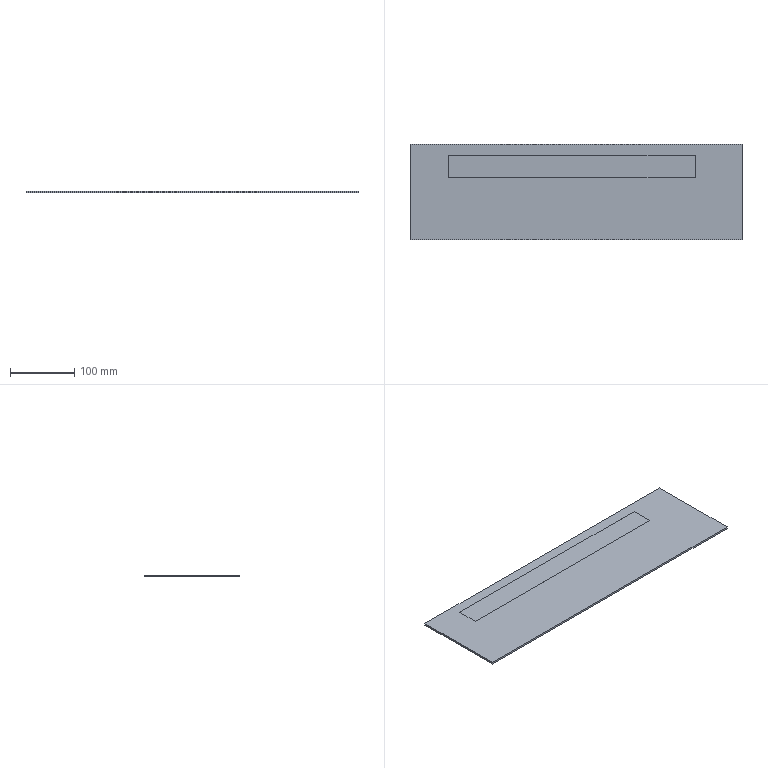Part | SolidWorks | features Extrusion 1, ICE 1 | 1 solid | 11 faces | box 515 x 148 x 3.01 mm | volume 228793 mm3 | plane 11
STEP:
#1=CARTESIAN_POINT('',(257.5,-74.,3.));
#2=VERTEX_POINT('',#1);
#3=CARTESIAN_POINT('',(257.5,74.,3.));
#4=VERTEX_POINT('',#3);
#5=CARTESIAN_POINT('',(257.5,74.,3.));
#6=DIRECTION('',(0.,1.,0.));
#7=VECTOR('',#6,1000.);
#8=LINE('',#5,#7);
#9=EDGE_CURVE('',#2,#4,#8,.T.);
#10=ORIENTED_EDGE('',*,*,#9,.T.);
#11=CARTESIAN_POINT('',(-257.5,74.,3.));
#12=VERTEX_POINT('',#11);
#13=CARTESIAN_POINT('',(-257.5,74.,3.));
#14=DIRECTION('',(-1.,0.,0.));
#15=VECTOR('',#14,1000.);
#16=LINE('',#13,#15);
#17=EDGE_CURVE('',#4,#12,#16,.T.);
#18=ORIENTED_EDGE('',*,*,#17,.T.);
#19=CARTESIAN_POINT('',(-257.5,-74.,3.));
#20=VERTEX_POINT('',#19);
#21=CARTESIAN_POINT('',(-257.5,74.,3.));
#22=DIRECTION('',(0.,-1.,0.));
#23=VECTOR('',#22,1000.);
#24=LINE('',#21,#23);
#25=EDGE_CURVE('',#12,#20,#24,.T.);
#26=ORIENTED_EDGE('',*,*,#25,.T.);
#27=CARTESIAN_POINT('',(-257.5,-74.,3.));
#28=DIRECTION('',(1.,0.,0.));
#29=VECTOR('',#28,1000.);
#30=LINE('',#27,#29);
#31=EDGE_CURVE('',#20,#2,#30,.T.);
#32=ORIENTED_EDGE('',*,*,#31,.T.);
#33=EDGE_LOOP('',(#10,#18,#26,#32));
#34=FACE_OUTER_BOUND('',#33,.T.);
#35=CARTESIAN_POINT('',(184.856,57.328,3.));
#36=VERTEX_POINT('',#35);
#37=CARTESIAN_POINT('',(-198.111,57.328,3.));
#38=VERTEX_POINT('',#37);
#39=CARTESIAN_POINT('',(184.856,57.328,3.));
#40=DIRECTION('',(-1.,0.,0.));
#41=VECTOR('',#40,1000.);
#42=LINE('',#39,#41);
#43=EDGE_CURVE('',#36,#38,#42,.T.);
#44=ORIENTED_EDGE('',*,*,#43,.F.);
#45=CARTESIAN_POINT('',(184.856,22.632,3.));
#46=VERTEX_POINT('',#45);
#47=CARTESIAN_POINT('',(184.856,57.328,3.));
#48=DIRECTION('',(0.,1.,0.));
#49=VECTOR('',#48,1000.);
#50=LINE('',#47,#49);
#51=EDGE_CURVE('',#46,#36,#50,.T.);
#52=ORIENTED_EDGE('',*,*,#51,.F.);
#53=CARTESIAN_POINT('',(-198.111,22.632,3.));
#54=VERTEX_POINT('',#53);
#55=CARTESIAN_POINT('',(184.856,22.632,3.));
#56=DIRECTION('',(1.,0.,0.));
#57=VECTOR('',#56,1000.);
#58=LINE('',#55,#57);
#59=EDGE_CURVE('',#54,#46,#58,.T.);
#60=ORIENTED_EDGE('',*,*,#59,.F.);
#61=CARTESIAN_POINT('',(-198.111,57.328,3.));
#62=DIRECTION('',(0.,-1.,0.));
#63=VECTOR('',#62,1000.);
#64=LINE('',#61,#63);
#65=EDGE_CURVE('',#38,#54,#64,.T.);
#66=ORIENTED_EDGE('',*,*,#65,.F.);
#67=EDGE_LOOP('',(#44,#52,#60,#66));
#68=FACE_BOUND('',#67,.T.);
#69=CARTESIAN_POINT('',(0.,0.,3.));
#70=DIRECTION('',(0.,0.,1.));
#71=DIRECTION('',(1.,0.,0.));
#72=AXIS2_PLACEMENT_3D('',#69,#70,#71);
#73=PLANE('',#72);
#74=ADVANCED_FACE('',(#34,#68),#73,.T.);
#75=CARTESIAN_POINT('',(257.5,-74.,0.));
#76=VERTEX_POINT('',#75);
#77=CARTESIAN_POINT('',(257.5,74.,0.));
#78=VERTEX_POINT('',#77);
#79=CARTESIAN_POINT('',(257.5,74.,0.));
#80=DIRECTION('',(0.,1.,0.));
#81=VECTOR('',#80,1000.);
#82=LINE('',#79,#81);
#83=EDGE_CURVE('',#76,#78,#82,.T.);
#84=ORIENTED_EDGE('',*,*,#83,.T.);
#85=CARTESIAN_POINT('',(257.5,74.,3.));
#86=DIRECTION('',(0.,0.,-1.));
#87=VECTOR('',#86,1000.);
#88=LINE('',#85,#87);
#89=EDGE_CURVE('',#4,#78,#88,.T.);
#90=ORIENTED_EDGE('',*,*,#89,.F.);
#91=ORIENTED_EDGE('',*,*,#9,.F.);
#92=CARTESIAN_POINT('',(257.5,-74.,3.));
#93=DIRECTION('',(0.,0.,-1.));
#94=VECTOR('',#93,1000.);
#95=LINE('',#92,#94);
#96=EDGE_CURVE('',#2,#76,#95,.T.);
#97=ORIENTED_EDGE('',*,*,#96,.T.);
#98=EDGE_LOOP('',(#84,#90,#91,#97));
#99=FACE_OUTER_BOUND('',#98,.T.);
#100=CARTESIAN_POINT('',(257.5,74.,3.));
#101=DIRECTION('',(-1.,0.,0.));
#102=DIRECTION('',(0.,0.,1.));
#103=AXIS2_PLACEMENT_3D('',#100,#101,#102);
#104=PLANE('',#103);
#105=ADVANCED_FACE('',(#99),#104,.F.);
#106=CARTESIAN_POINT('',(-257.5,74.,0.));
#107=VERTEX_POINT('',#106);
#108=CARTESIAN_POINT('',(-257.5,74.,0.));
#109=DIRECTION('',(-1.,0.,0.));
#110=VECTOR('',#109,1000.);
#111=LINE('',#108,#110);
#112=EDGE_CURVE('',#78,#107,#111,.T.);
#113=ORIENTED_EDGE('',*,*,#112,.T.);
#114=CARTESIAN_POINT('',(-257.5,74.,3.));
#115=DIRECTION('',(0.,0.,-1.));
#116=VECTOR('',#115,1000.);
#117=LINE('',#114,#116);
#118=EDGE_CURVE('',#12,#107,#117,.T.);
#119=ORIENTED_EDGE('',*,*,#118,.F.);
#120=ORIENTED_EDGE('',*,*,#17,.F.);
#121=ORIENTED_EDGE('',*,*,#89,.T.);
#122=EDGE_LOOP('',(#113,#119,#120,#121));
#123=FACE_OUTER_BOUND('',#122,.T.);
#124=CARTESIAN_POINT('',(-257.5,74.,3.));
#125=DIRECTION('',(0.,-1.,0.));
#126=DIRECTION('',(0.,0.,-1.));
#127=AXIS2_PLACEMENT_3D('',#124,#125,#126);
#128=PLANE('',#127);
#129=ADVANCED_FACE('',(#123),#128,.F.);
#130=CARTESIAN_POINT('',(-257.5,-74.,0.));
#131=VERTEX_POINT('',#130);
#132=CARTESIAN_POINT('',(-257.5,74.,0.));
#133=DIRECTION('',(0.,-1.,0.));
#134=VECTOR('',#133,1000.);
#135=LINE('',#132,#134);
#136=EDGE_CURVE('',#107,#131,#135,.T.);
#137=ORIENTED_EDGE('',*,*,#136,.T.);
#138=CARTESIAN_POINT('',(-257.5,-74.,3.));
#139=DIRECTION('',(0.,0.,-1.));
#140=VECTOR('',#139,1000.);
#141=LINE('',#138,#140);
#142=EDGE_CURVE('',#20,#131,#141,.T.);
#143=ORIENTED_EDGE('',*,*,#142,.F.);
#144=ORIENTED_EDGE('',*,*,#25,.F.);
#145=ORIENTED_EDGE('',*,*,#118,.T.);
#146=EDGE_LOOP('',(#137,#143,#144,#145));
#147=FACE_OUTER_BOUND('',#146,.T.);
#148=CARTESIAN_POINT('',(-257.5,74.,3.));
#149=DIRECTION('',(1.,0.,0.));
#150=DIRECTION('',(0.,0.,-1.));
#151=AXIS2_PLACEMENT_3D('',#148,#149,#150);
#152=PLANE('',#151);
#153=ADVANCED_FACE('',(#147),#152,.F.);
#154=CARTESIAN_POINT('',(-257.5,-74.,0.));
#155=DIRECTION('',(1.,0.,0.));
#156=VECTOR('',#155,1000.);
#157=LINE('',#154,#156);
#158=EDGE_CURVE('',#131,#76,#157,.T.);
#159=ORIENTED_EDGE('',*,*,#158,.T.);
#160=ORIENTED_EDGE('',*,*,#96,.F.);
#161=ORIENTED_EDGE('',*,*,#31,.F.);
#162=ORIENTED_EDGE('',*,*,#142,.T.);
#163=EDGE_LOOP('',(#159,#160,#161,#162));
#164=FACE_OUTER_BOUND('',#163,.T.);
#165=CARTESIAN_POINT('',(-257.5,-74.,3.));
#166=DIRECTION('',(0.,1.,0.));
#167=DIRECTION('',(0.,0.,1.));
#168=AXIS2_PLACEMENT_3D('',#165,#166,#167);
#169=PLANE('',#168);
#170=ADVANCED_FACE('',(#164),#169,.F.);
#171=ORIENTED_EDGE('',*,*,#83,.F.);
#172=ORIENTED_EDGE('',*,*,#158,.F.);
#173=ORIENTED_EDGE('',*,*,#136,.F.);
#174=ORIENTED_EDGE('',*,*,#112,.F.);
#175=EDGE_LOOP('',(#171,#172,#173,#174));
#176=FACE_OUTER_BOUND('',#175,.T.);
#177=CARTESIAN_POINT('',(0.,0.,0.));
#178=DIRECTION('',(0.,0.,1.));
#179=DIRECTION('',(1.,0.,0.));
#180=AXIS2_PLACEMENT_3D('',#177,#178,#179);
#181=PLANE('',#180);
#182=ADVANCED_FACE('',(#176),#181,.F.);
#183=ORIENTED_EDGE('',*,*,#51,.T.);
#184=CARTESIAN_POINT('',(184.856,57.328,3.01));
#185=VERTEX_POINT('',#184);
#186=CARTESIAN_POINT('',(184.856,57.328,3.01));
#187=DIRECTION('',(0.,0.,-1.));
#188=VECTOR('',#187,1000.);
#189=LINE('',#186,#188);
#190=EDGE_CURVE('',#185,#36,#189,.T.);
#191=ORIENTED_EDGE('',*,*,#190,.F.);
#192=CARTESIAN_POINT('',(184.856,22.632,3.01));
#193=VERTEX_POINT('',#192);
#194=CARTESIAN_POINT('',(184.856,57.328,3.01));
#195=DIRECTION('',(0.,1.,0.));
#196=VECTOR('',#195,1000.);
#197=LINE('',#194,#196);
#198=EDGE_CURVE('',#193,#185,#197,.T.);
#199=ORIENTED_EDGE('',*,*,#198,.F.);
#200=CARTESIAN_POINT('',(184.856,22.632,3.01));
#201=DIRECTION('',(0.,0.,-1.));
#202=VECTOR('',#201,1000.);
#203=LINE('',#200,#202);
#204=EDGE_CURVE('',#193,#46,#203,.T.);
#205=ORIENTED_EDGE('',*,*,#204,.T.);
#206=EDGE_LOOP('',(#183,#191,#199,#205));
#207=FACE_OUTER_BOUND('',#206,.T.);
#208=CARTESIAN_POINT('',(184.856,57.328,3.01));
#209=DIRECTION('',(-1.,0.,0.));
#210=DIRECTION('',(0.,0.,1.));
#211=AXIS2_PLACEMENT_3D('',#208,#209,#210);
#212=PLANE('',#211);
#213=ADVANCED_FACE('',(#207),#212,.F.);
#214=ORIENTED_EDGE('',*,*,#43,.T.);
#215=CARTESIAN_POINT('',(-198.111,57.328,3.01));
#216=VERTEX_POINT('',#215);
#217=CARTESIAN_POINT('',(-198.111,57.328,3.01));
#218=DIRECTION('',(0.,0.,-1.));
#219=VECTOR('',#218,1000.);
#220=LINE('',#217,#219);
#221=EDGE_CURVE('',#216,#38,#220,.T.);
#222=ORIENTED_EDGE('',*,*,#221,.F.);
#223=CARTESIAN_POINT('',(184.856,57.328,3.01));
#224=DIRECTION('',(-1.,0.,0.));
#225=VECTOR('',#224,1000.);
#226=LINE('',#223,#225);
#227=EDGE_CURVE('',#185,#216,#226,.T.);
#228=ORIENTED_EDGE('',*,*,#227,.F.);
#229=ORIENTED_EDGE('',*,*,#190,.T.);
#230=EDGE_LOOP('',(#214,#222,#228,#229));
#231=FACE_OUTER_BOUND('',#230,.T.);
#232=CARTESIAN_POINT('',(184.856,57.328,3.01));
#233=DIRECTION('',(0.,-1.,0.));
#234=DIRECTION('',(0.,0.,-1.));
#235=AXIS2_PLACEMENT_3D('',#232,#233,#234);
#236=PLANE('',#235);
#237=ADVANCED_FACE('',(#231),#236,.F.);
#238=ORIENTED_EDGE('',*,*,#65,.T.);
#239=CARTESIAN_POINT('',(-198.111,22.632,3.01));
#240=VERTEX_POINT('',#239);
#241=CARTESIAN_POINT('',(-198.111,22.632,3.01));
#242=DIRECTION('',(0.,0.,-1.));
#243=VECTOR('',#242,1000.);
#244=LINE('',#241,#243);
#245=EDGE_CURVE('',#240,#54,#244,.T.);
#246=ORIENTED_EDGE('',*,*,#245,.F.);
#247=CARTESIAN_POINT('',(-198.111,57.328,3.01));
#248=DIRECTION('',(0.,-1.,0.));
#249=VECTOR('',#248,1000.);
#250=LINE('',#247,#249);
#251=EDGE_CURVE('',#216,#240,#250,.T.);
#252=ORIENTED_EDGE('',*,*,#251,.F.);
#253=ORIENTED_EDGE('',*,*,#221,.T.);
#254=EDGE_LOOP('',(#238,#246,#252,#253));
#255=FACE_OUTER_BOUND('',#254,.T.);
#256=CARTESIAN_POINT('',(-198.111,57.328,3.01));
#257=DIRECTION('',(1.,0.,0.));
#258=DIRECTION('',(0.,0.,-1.));
#259=AXIS2_PLACEMENT_3D('',#256,#257,#258);
#260=PLANE('',#259);
#261=ADVANCED_FACE('',(#255),#260,.F.);
#262=ORIENTED_EDGE('',*,*,#59,.T.);
#263=ORIENTED_EDGE('',*,*,#204,.F.);
#264=CARTESIAN_POINT('',(184.856,22.632,3.01));
#265=DIRECTION('',(1.,0.,0.));
#266=VECTOR('',#265,1000.);
#267=LINE('',#264,#266);
#268=EDGE_CURVE('',#240,#193,#267,.T.);
#269=ORIENTED_EDGE('',*,*,#268,.F.);
#270=ORIENTED_EDGE('',*,*,#245,.T.);
#271=EDGE_LOOP('',(#262,#263,#269,#270));
#272=FACE_OUTER_BOUND('',#271,.T.);
#273=CARTESIAN_POINT('',(184.856,22.632,3.01));
#274=DIRECTION('',(0.,1.,0.));
#275=DIRECTION('',(0.,0.,1.));
#276=AXIS2_PLACEMENT_3D('',#273,#274,#275);
#277=PLANE('',#276);
#278=ADVANCED_FACE('',(#272),#277,.F.);
#279=ORIENTED_EDGE('',*,*,#198,.T.);
#280=ORIENTED_EDGE('',*,*,#227,.T.);
#281=ORIENTED_EDGE('',*,*,#251,.T.);
#282=ORIENTED_EDGE('',*,*,#268,.T.);
#283=EDGE_LOOP('',(#279,#280,#281,#282));
#284=FACE_OUTER_BOUND('',#283,.T.);
#285=CARTESIAN_POINT('',(0.,0.,3.01));
#286=DIRECTION('',(0.,0.,-1.));
#287=DIRECTION('',(-1.,0.,0.));
#288=AXIS2_PLACEMENT_3D('',#285,#286,#287);
#289=PLANE('',#288);
#290=ADVANCED_FACE('',(#284),#289,.F.);
#291=CLOSED_SHELL('',(#74,#105,#129,#153,#170,#182,#213,#237,#261,#278,#290));
#292=MANIFOLD_SOLID_BREP('',#291);
#293=CARTESIAN_POINT('',(0.,0.,0.));
#294=DIRECTION('',(0.,0.,1.));
#295=DIRECTION('',(1.,0.,0.));
#296=AXIS2_PLACEMENT_3D('',#293,#294,#295);
#297=(LENGTH_UNIT()NAMED_UNIT(*)SI_UNIT(.MILLI.,.METRE.));
#298=UNCERTAINTY_MEASURE_WITH_UNIT(LENGTH_MEASURE(0.00001),#297,'','');
#299=(NAMED_UNIT(*)PLANE_ANGLE_UNIT()SI_UNIT($,.RADIAN.));
#300=(NAMED_UNIT(*)SI_UNIT($,.STERADIAN.)SOLID_ANGLE_UNIT());
#301=(GEOMETRIC_REPRESENTATION_CONTEXT(3)GLOBAL_UNCERTAINTY_ASSIGNED_CONTEXT((#298))GLOBAL_UNIT_ASSIGNED_CONTEXT((#297,#299,#300))REPRESENTATION_CONTEXT('',''));
#302=ADVANCED_BREP_SHAPE_REPRESENTATION('',(#292,#296),#301);